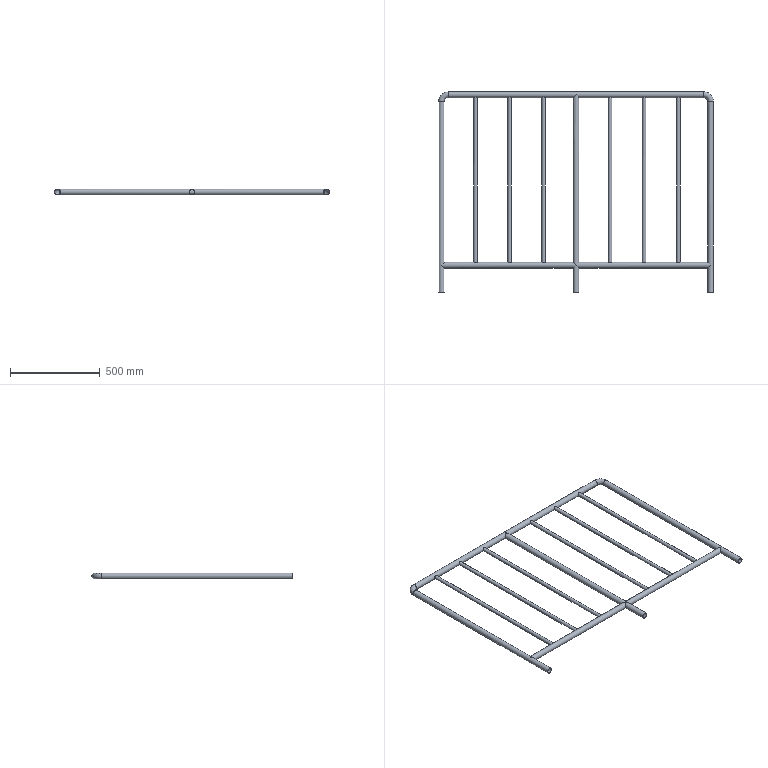Part | STEP file | 304 guardrail 1500X1100-B_Default<As Machined> | 14 solids | 56 faces | box 1532 x 1116 x 32 mm | volume 1222525 mm3 | cylinder 41 | plane 11 | torus 4 | commonest cylinder face diameters 32 x23 18 x6 20 x6 29 x6